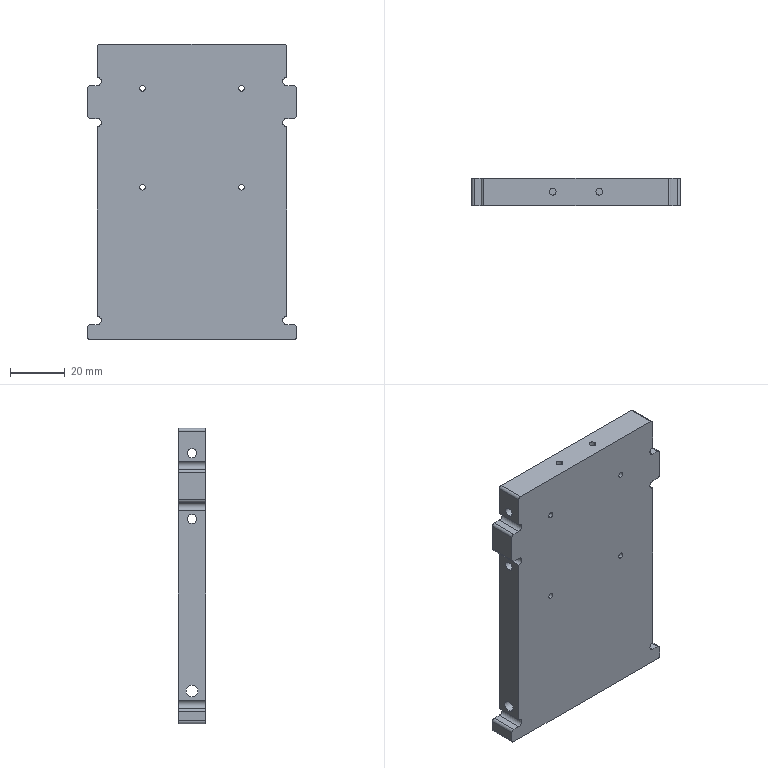Part | SolidWorks | features HoleWzd 5, Fillet 2, Extrusion 1, ICE 1 | 1 solid | 127 faces | box 76 x 10 x 107.5 mm | volume 24777 mm3 | cylinder 76 | plane 51 | commonest cylinder face diameters 3 x38 2 x10 2.05 x8 3.3 x8 2.5 x4 4.2 x4